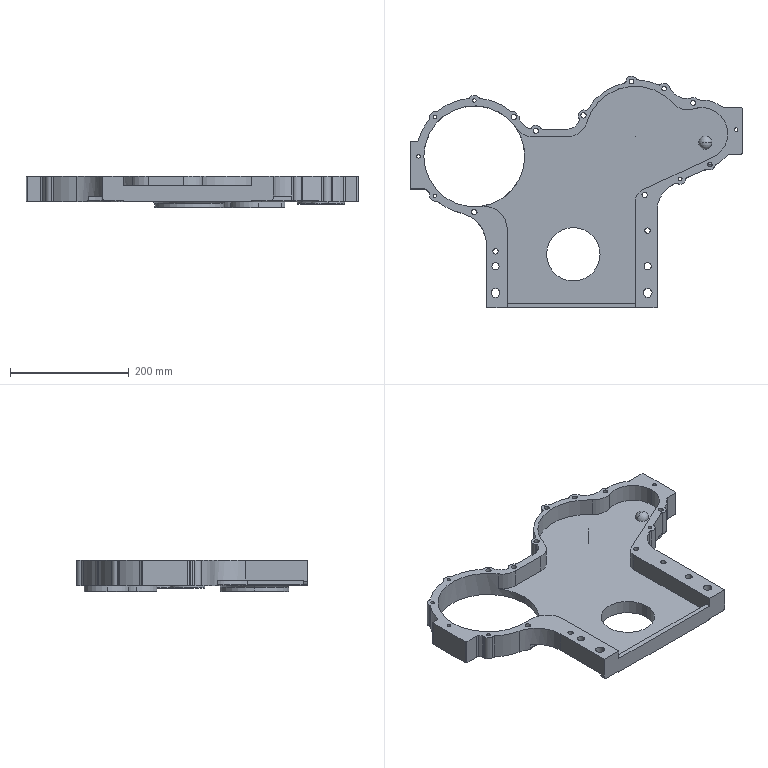Part | SolidWorks | features BaseBody 3 | 3 solids | 242 faces | box 558.999 x 390 x 53.5 mm | volume 2295511 mm3 | cylinder 162 | plane 52 | torus 24 | sphere 4 | commonest cylinder face diameters 8 x42 6 x16 9 x14 18 x12 7 x8 196 x6